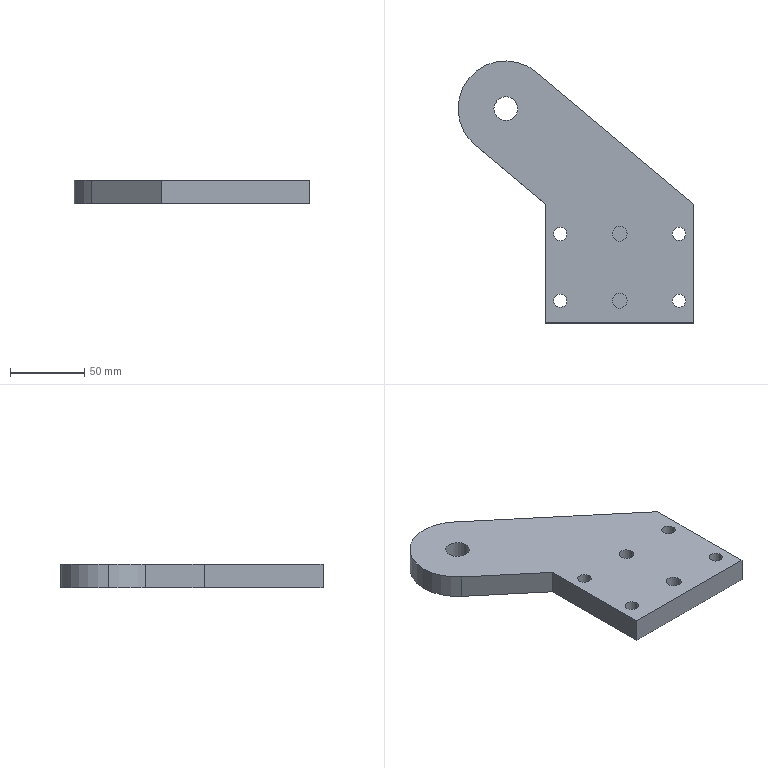Part | SolidWorks | features BaseBody 1 | 1 solid | 25 faces | box 158.743 x 176.419 x 16 mm | volume 247944 mm3 | cylinder 16 | plane 9 | commonest cylinder face diameters 9 x8 10.01 x4 16 x2 64.28 x2
STEP:
#1=CARTESIAN_POINT('',(-35.5,85.,-32.879));
#2=VERTEX_POINT('',#1);
#3=CARTESIAN_POINT('',(-44.5,85.,-32.879));
#4=VERTEX_POINT('',#3);
#5=CARTESIAN_POINT('',(-40.,85.,-32.879));
#6=DIRECTION('',(0.,0.,-1.));
#7=DIRECTION('',(1.,0.,0.));
#8=AXIS2_PLACEMENT_3D('',#5,#6,#7);
#9=CIRCLE('',#8,4.5);
#10=EDGE_CURVE('',#2,#4,#9,.T.);
#11=ORIENTED_EDGE('',*,*,#10,.T.);
#12=CARTESIAN_POINT('',(-44.5,85.,-16.879));
#13=VERTEX_POINT('',#12);
#14=CARTESIAN_POINT('',(-44.5,85.,-32.88));
#15=DIRECTION('',(0.,0.,1.));
#16=VECTOR('',#15,1000.);
#17=LINE('',#14,#16);
#18=EDGE_CURVE('',#4,#13,#17,.T.);
#19=ORIENTED_EDGE('',*,*,#18,.T.);
#20=CARTESIAN_POINT('',(-35.5,85.,-16.879));
#21=VERTEX_POINT('',#20);
#22=CARTESIAN_POINT('',(-40.,85.,-16.879));
#23=DIRECTION('',(0.,0.,-1.));
#24=DIRECTION('',(1.,0.,0.));
#25=AXIS2_PLACEMENT_3D('',#22,#23,#24);
#26=CIRCLE('',#25,4.5);
#27=EDGE_CURVE('',#21,#13,#26,.T.);
#28=ORIENTED_EDGE('',*,*,#27,.F.);
#29=CARTESIAN_POINT('',(-35.5,85.,-32.88));
#30=DIRECTION('',(0.,0.,1.));
#31=VECTOR('',#30,1000.);
#32=LINE('',#29,#31);
#33=EDGE_CURVE('',#2,#21,#32,.T.);
#34=ORIENTED_EDGE('',*,*,#33,.F.);
#35=EDGE_LOOP('',(#11,#19,#28,#34));
#36=FACE_OUTER_BOUND('',#35,.T.);
#37=CARTESIAN_POINT('',(-40.,85.,-32.88));
#38=DIRECTION('',(0.,0.,1.));
#39=DIRECTION('',(1.,0.,0.));
#40=AXIS2_PLACEMENT_3D('',#37,#38,#39);
#41=CYLINDRICAL_SURFACE('',#40,4.5);
#42=ADVANCED_FACE('',(#36),#41,.F.);
#43=CARTESIAN_POINT('',(-97.263,189.658,-16.879));
#44=VERTEX_POINT('',#43);
#45=CARTESIAN_POINT('',(-108.743,214.279,-16.879));
#46=VERTEX_POINT('',#45);
#47=CARTESIAN_POINT('',(-76.603,214.279,-16.879));
#48=DIRECTION('',(0.,0.,-1.));
#49=DIRECTION('',(-1.,0.,0.));
#50=AXIS2_PLACEMENT_3D('',#47,#48,#49);
#51=CIRCLE('',#50,32.14);
#52=EDGE_CURVE('',#44,#46,#51,.T.);
#53=ORIENTED_EDGE('',*,*,#52,.T.);
#54=CARTESIAN_POINT('',(-108.743,214.279,-32.879));
#55=VERTEX_POINT('',#54);
#56=CARTESIAN_POINT('',(-108.743,214.279,-16.879));
#57=DIRECTION('',(0.,0.,-1.));
#58=VECTOR('',#57,1000.);
#59=LINE('',#56,#58);
#60=EDGE_CURVE('',#46,#55,#59,.T.);
#61=ORIENTED_EDGE('',*,*,#60,.T.);
#62=CARTESIAN_POINT('',(-97.263,189.658,-32.879));
#63=VERTEX_POINT('',#62);
#64=CARTESIAN_POINT('',(-76.603,214.279,-32.879));
#65=DIRECTION('',(0.,0.,1.));
#66=DIRECTION('',(-1.,0.,0.));
#67=AXIS2_PLACEMENT_3D('',#64,#65,#66);
#68=CIRCLE('',#67,32.14);
#69=EDGE_CURVE('',#55,#63,#68,.T.);
#70=ORIENTED_EDGE('',*,*,#69,.T.);
#71=CARTESIAN_POINT('',(-97.263,189.658,-16.879));
#72=DIRECTION('',(0.,0.,1.));
#73=VECTOR('',#72,1000.);
#74=LINE('',#71,#73);
#75=EDGE_CURVE('',#63,#44,#74,.T.);
#76=ORIENTED_EDGE('',*,*,#75,.T.);
#77=EDGE_LOOP('',(#53,#61,#70,#76));
#78=FACE_OUTER_BOUND('',#77,.T.);
#79=CARTESIAN_POINT('',(-76.603,214.279,-16.879));
#80=DIRECTION('',(0.,0.,-1.));
#81=DIRECTION('',(-1.,0.,0.));
#82=AXIS2_PLACEMENT_3D('',#79,#80,#81);
#83=CYLINDRICAL_SURFACE('',#82,32.14);
#84=ADVANCED_FACE('',(#78),#83,.T.);
#85=CARTESIAN_POINT('',(44.5,130.,-32.879));
#86=VERTEX_POINT('',#85);
#87=CARTESIAN_POINT('',(35.5,130.,-32.879));
#88=VERTEX_POINT('',#87);
#89=CARTESIAN_POINT('',(40.,130.,-32.879));
#90=DIRECTION('',(0.,0.,-1.));
#91=DIRECTION('',(1.,0.,0.));
#92=AXIS2_PLACEMENT_3D('',#89,#90,#91);
#93=CIRCLE('',#92,4.5);
#94=EDGE_CURVE('',#86,#88,#93,.T.);
#95=ORIENTED_EDGE('',*,*,#94,.T.);
#96=CARTESIAN_POINT('',(35.5,130.,-16.879));
#97=VERTEX_POINT('',#96);
#98=CARTESIAN_POINT('',(35.5,130.,-32.88));
#99=DIRECTION('',(0.,0.,1.));
#100=VECTOR('',#99,1000.);
#101=LINE('',#98,#100);
#102=EDGE_CURVE('',#88,#97,#101,.T.);
#103=ORIENTED_EDGE('',*,*,#102,.T.);
#104=CARTESIAN_POINT('',(44.5,130.,-16.879));
#105=VERTEX_POINT('',#104);
#106=CARTESIAN_POINT('',(40.,130.,-16.879));
#107=DIRECTION('',(0.,0.,-1.));
#108=DIRECTION('',(1.,0.,0.));
#109=AXIS2_PLACEMENT_3D('',#106,#107,#108);
#110=CIRCLE('',#109,4.5);
#111=EDGE_CURVE('',#105,#97,#110,.T.);
#112=ORIENTED_EDGE('',*,*,#111,.F.);
#113=CARTESIAN_POINT('',(44.5,130.,-32.88));
#114=DIRECTION('',(0.,0.,1.));
#115=VECTOR('',#114,1000.);
#116=LINE('',#113,#115);
#117=EDGE_CURVE('',#86,#105,#116,.T.);
#118=ORIENTED_EDGE('',*,*,#117,.F.);
#119=EDGE_LOOP('',(#95,#103,#112,#118));
#120=FACE_OUTER_BOUND('',#119,.T.);
#121=CARTESIAN_POINT('',(40.,130.,-32.88));
#122=DIRECTION('',(0.,0.,1.));
#123=DIRECTION('',(1.,0.,0.));
#124=AXIS2_PLACEMENT_3D('',#121,#122,#123);
#125=CYLINDRICAL_SURFACE('',#124,4.5);
#126=ADVANCED_FACE('',(#120),#125,.F.);
#127=CARTESIAN_POINT('',(44.5,85.,-32.879));
#128=VERTEX_POINT('',#127);
#129=CARTESIAN_POINT('',(35.5,85.,-32.879));
#130=VERTEX_POINT('',#129);
#131=CARTESIAN_POINT('',(40.,85.,-32.879));
#132=DIRECTION('',(0.,0.,-1.));
#133=DIRECTION('',(1.,0.,0.));
#134=AXIS2_PLACEMENT_3D('',#131,#132,#133);
#135=CIRCLE('',#134,4.5);
#136=EDGE_CURVE('',#128,#130,#135,.T.);
#137=ORIENTED_EDGE('',*,*,#136,.T.);
#138=CARTESIAN_POINT('',(35.5,85.,-16.879));
#139=VERTEX_POINT('',#138);
#140=CARTESIAN_POINT('',(35.5,85.,-32.88));
#141=DIRECTION('',(0.,0.,1.));
#142=VECTOR('',#141,1000.);
#143=LINE('',#140,#142);
#144=EDGE_CURVE('',#130,#139,#143,.T.);
#145=ORIENTED_EDGE('',*,*,#144,.T.);
#146=CARTESIAN_POINT('',(44.5,85.,-16.879));
#147=VERTEX_POINT('',#146);
#148=CARTESIAN_POINT('',(40.,85.,-16.879));
#149=DIRECTION('',(0.,0.,-1.));
#150=DIRECTION('',(1.,0.,0.));
#151=AXIS2_PLACEMENT_3D('',#148,#149,#150);
#152=CIRCLE('',#151,4.5);
#153=EDGE_CURVE('',#147,#139,#152,.T.);
#154=ORIENTED_EDGE('',*,*,#153,.F.);
#155=CARTESIAN_POINT('',(44.5,85.,-32.88));
#156=DIRECTION('',(0.,0.,1.));
#157=VECTOR('',#156,1000.);
#158=LINE('',#155,#157);
#159=EDGE_CURVE('',#128,#147,#158,.T.);
#160=ORIENTED_EDGE('',*,*,#159,.F.);
#161=EDGE_LOOP('',(#137,#145,#154,#160));
#162=FACE_OUTER_BOUND('',#161,.T.);
#163=CARTESIAN_POINT('',(40.,85.,-32.88));
#164=DIRECTION('',(0.,0.,1.));
#165=DIRECTION('',(1.,0.,0.));
#166=AXIS2_PLACEMENT_3D('',#163,#164,#165);
#167=CYLINDRICAL_SURFACE('',#166,4.5);
#168=ADVANCED_FACE('',(#162),#167,.F.);
#169=CARTESIAN_POINT('',(-35.5,130.,-32.879));
#170=VERTEX_POINT('',#169);
#171=CARTESIAN_POINT('',(-44.5,130.,-32.879));
#172=VERTEX_POINT('',#171);
#173=CARTESIAN_POINT('',(-40.,130.,-32.879));
#174=DIRECTION('',(0.,0.,-1.));
#175=DIRECTION('',(1.,0.,0.));
#176=AXIS2_PLACEMENT_3D('',#173,#174,#175);
#177=CIRCLE('',#176,4.5);
#178=EDGE_CURVE('',#170,#172,#177,.T.);
#179=ORIENTED_EDGE('',*,*,#178,.T.);
#180=CARTESIAN_POINT('',(-44.5,130.,-16.879));
#181=VERTEX_POINT('',#180);
#182=CARTESIAN_POINT('',(-44.5,130.,-32.88));
#183=DIRECTION('',(0.,0.,1.));
#184=VECTOR('',#183,1000.);
#185=LINE('',#182,#184);
#186=EDGE_CURVE('',#172,#181,#185,.T.);
#187=ORIENTED_EDGE('',*,*,#186,.T.);
#188=CARTESIAN_POINT('',(-35.5,130.,-16.879));
#189=VERTEX_POINT('',#188);
#190=CARTESIAN_POINT('',(-40.,130.,-16.879));
#191=DIRECTION('',(0.,0.,-1.));
#192=DIRECTION('',(1.,0.,0.));
#193=AXIS2_PLACEMENT_3D('',#190,#191,#192);
#194=CIRCLE('',#193,4.5);
#195=EDGE_CURVE('',#189,#181,#194,.T.);
#196=ORIENTED_EDGE('',*,*,#195,.F.);
#197=CARTESIAN_POINT('',(-35.5,130.,-32.88));
#198=DIRECTION('',(0.,0.,1.));
#199=VECTOR('',#198,1000.);
#200=LINE('',#197,#199);
#201=EDGE_CURVE('',#170,#189,#200,.T.);
#202=ORIENTED_EDGE('',*,*,#201,.F.);
#203=EDGE_LOOP('',(#179,#187,#196,#202));
#204=FACE_OUTER_BOUND('',#203,.T.);
#205=CARTESIAN_POINT('',(-40.,130.,-32.88));
#206=DIRECTION('',(0.,0.,1.));
#207=DIRECTION('',(1.,0.,0.));
#208=AXIS2_PLACEMENT_3D('',#205,#206,#207);
#209=CYLINDRICAL_SURFACE('',#208,4.5);
#210=ADVANCED_FACE('',(#204),#209,.F.);
#211=CARTESIAN_POINT('',(-68.603,214.279,-32.879));
#212=VERTEX_POINT('',#211);
#213=CARTESIAN_POINT('',(-84.603,214.279,-32.879));
#214=VERTEX_POINT('',#213);
#215=CARTESIAN_POINT('',(-76.603,214.279,-32.879));
#216=DIRECTION('',(0.,0.,-1.));
#217=DIRECTION('',(1.,0.,0.));
#218=AXIS2_PLACEMENT_3D('',#215,#216,#217);
#219=CIRCLE('',#218,8.);
#220=EDGE_CURVE('',#212,#214,#219,.T.);
#221=ORIENTED_EDGE('',*,*,#220,.T.);
#222=CARTESIAN_POINT('',(-84.603,214.279,-16.879));
#223=VERTEX_POINT('',#222);
#224=CARTESIAN_POINT('',(-84.603,214.279,-32.88));
#225=DIRECTION('',(0.,0.,1.));
#226=VECTOR('',#225,1000.);
#227=LINE('',#224,#226);
#228=EDGE_CURVE('',#214,#223,#227,.T.);
#229=ORIENTED_EDGE('',*,*,#228,.T.);
#230=CARTESIAN_POINT('',(-68.603,214.279,-16.879));
#231=VERTEX_POINT('',#230);
#232=CARTESIAN_POINT('',(-76.603,214.279,-16.879));
#233=DIRECTION('',(0.,0.,-1.));
#234=DIRECTION('',(1.,0.,0.));
#235=AXIS2_PLACEMENT_3D('',#232,#233,#234);
#236=CIRCLE('',#235,8.);
#237=EDGE_CURVE('',#231,#223,#236,.T.);
#238=ORIENTED_EDGE('',*,*,#237,.F.);
#239=CARTESIAN_POINT('',(-68.603,214.279,-32.88));
#240=DIRECTION('',(0.,0.,1.));
#241=VECTOR('',#240,1000.);
#242=LINE('',#239,#241);
#243=EDGE_CURVE('',#212,#231,#242,.T.);
#244=ORIENTED_EDGE('',*,*,#243,.F.);
#245=EDGE_LOOP('',(#221,#229,#238,#244));
#246=FACE_OUTER_BOUND('',#245,.T.);
#247=CARTESIAN_POINT('',(-76.603,214.279,-32.88));
#248=DIRECTION('',(0.,0.,1.));
#249=DIRECTION('',(1.,0.,0.));
#250=AXIS2_PLACEMENT_3D('',#247,#248,#249);
#251=CYLINDRICAL_SURFACE('',#250,8.);
#252=ADVANCED_FACE('',(#246),#251,.F.);
#253=CARTESIAN_POINT('',(-5.005,130.,-26.879));
#254=VERTEX_POINT('',#253);
#255=CARTESIAN_POINT('',(5.005,130.,-26.879));
#256=VERTEX_POINT('',#255);
#257=CARTESIAN_POINT('',(0.,130.,-26.879));
#258=DIRECTION('',(0.,0.,1.));
#259=DIRECTION('',(1.,0.,0.));
#260=AXIS2_PLACEMENT_3D('',#257,#258,#259);
#261=CIRCLE('',#260,5.005);
#262=EDGE_CURVE('',#254,#256,#261,.T.);
#263=ORIENTED_EDGE('',*,*,#262,.F.);
#264=CARTESIAN_POINT('',(-5.005,130.,-16.879));
#265=VERTEX_POINT('',#264);
#266=CARTESIAN_POINT('',(-5.005,130.,-26.879));
#267=DIRECTION('',(0.,0.,1.));
#268=VECTOR('',#267,1000.);
#269=LINE('',#266,#268);
#270=EDGE_CURVE('',#254,#265,#269,.T.);
#271=ORIENTED_EDGE('',*,*,#270,.T.);
#272=CARTESIAN_POINT('',(5.005,130.,-16.879));
#273=VERTEX_POINT('',#272);
#274=CARTESIAN_POINT('',(0.,130.,-16.879));
#275=DIRECTION('',(0.,0.,-1.));
#276=DIRECTION('',(1.,0.,0.));
#277=AXIS2_PLACEMENT_3D('',#274,#275,#276);
#278=CIRCLE('',#277,5.005);
#279=EDGE_CURVE('',#273,#265,#278,.T.);
#280=ORIENTED_EDGE('',*,*,#279,.F.);
#281=CARTESIAN_POINT('',(5.005,130.,-26.879));
#282=DIRECTION('',(0.,0.,1.));
#283=VECTOR('',#282,1000.);
#284=LINE('',#281,#283);
#285=EDGE_CURVE('',#256,#273,#284,.T.);
#286=ORIENTED_EDGE('',*,*,#285,.F.);
#287=EDGE_LOOP('',(#263,#271,#280,#286));
#288=FACE_OUTER_BOUND('',#287,.T.);
#289=CARTESIAN_POINT('',(0.,130.,-26.879));
#290=DIRECTION('',(0.,0.,1.));
#291=DIRECTION('',(1.,0.,0.));
#292=AXIS2_PLACEMENT_3D('',#289,#290,#291);
#293=CYLINDRICAL_SURFACE('',#292,5.005);
#294=ADVANCED_FACE('',(#288),#293,.F.);
#295=CARTESIAN_POINT('',(-5.005,85.,-26.879));
#296=VERTEX_POINT('',#295);
#297=CARTESIAN_POINT('',(5.005,85.,-26.879));
#298=VERTEX_POINT('',#297);
#299=CARTESIAN_POINT('',(0.,85.,-26.879));
#300=DIRECTION('',(0.,0.,1.));
#301=DIRECTION('',(1.,0.,0.));
#302=AXIS2_PLACEMENT_3D('',#299,#300,#301);
#303=CIRCLE('',#302,5.005);
#304=EDGE_CURVE('',#296,#298,#303,.T.);
#305=ORIENTED_EDGE('',*,*,#304,.F.);
#306=CARTESIAN_POINT('',(-5.005,85.,-16.879));
#307=VERTEX_POINT('',#306);
#308=CARTESIAN_POINT('',(-5.005,85.,-26.879));
#309=DIRECTION('',(0.,0.,1.));
#310=VECTOR('',#309,1000.);
#311=LINE('',#308,#310);
#312=EDGE_CURVE('',#296,#307,#311,.T.);
#313=ORIENTED_EDGE('',*,*,#312,.T.);
#314=CARTESIAN_POINT('',(5.005,85.,-16.879));
#315=VERTEX_POINT('',#314);
#316=CARTESIAN_POINT('',(0.,85.,-16.879));
#317=DIRECTION('',(0.,0.,-1.));
#318=DIRECTION('',(1.,0.,0.));
#319=AXIS2_PLACEMENT_3D('',#316,#317,#318);
#320=CIRCLE('',#319,5.005);
#321=EDGE_CURVE('',#315,#307,#320,.T.);
#322=ORIENTED_EDGE('',*,*,#321,.F.);
#323=CARTESIAN_POINT('',(5.005,85.,-26.879));
#324=DIRECTION('',(0.,0.,1.));
#325=VECTOR('',#324,1000.);
#326=LINE('',#323,#325);
#327=EDGE_CURVE('',#298,#315,#326,.T.);
#328=ORIENTED_EDGE('',*,*,#327,.F.);
#329=EDGE_LOOP('',(#305,#313,#322,#328));
#330=FACE_OUTER_BOUND('',#329,.T.);
#331=CARTESIAN_POINT('',(0.,85.,-26.879));
#332=DIRECTION('',(0.,0.,1.));
#333=DIRECTION('',(1.,0.,0.));
#334=AXIS2_PLACEMENT_3D('',#331,#332,#333);
#335=CYLINDRICAL_SURFACE('',#334,5.005);
#336=ADVANCED_FACE('',(#330),#335,.F.);
#337=ORIENTED_EDGE('',*,*,#10,.F.);
#338=CARTESIAN_POINT('',(-40.,85.,-32.879));
#339=DIRECTION('',(0.,0.,-1.));
#340=DIRECTION('',(1.,0.,0.));
#341=AXIS2_PLACEMENT_3D('',#338,#339,#340);
#342=CIRCLE('',#341,4.5);
#343=EDGE_CURVE('',#4,#2,#342,.T.);
#344=ORIENTED_EDGE('',*,*,#343,.F.);
#345=EDGE_LOOP('',(#337,#344));
#346=FACE_BOUND('',#345,.T.);
#347=CARTESIAN_POINT('',(-50.,70.,-32.879));
#348=VERTEX_POINT('',#347);
#349=CARTESIAN_POINT('',(50.,70.,-32.879));
#350=VERTEX_POINT('',#349);
#351=CARTESIAN_POINT('',(-76.603,70.,-32.879));
#352=DIRECTION('',(1.,0.,0.));
#353=VECTOR('',#352,1000.);
#354=LINE('',#351,#353);
#355=EDGE_CURVE('',#348,#350,#354,.T.);
#356=ORIENTED_EDGE('',*,*,#355,.F.);
#357=CARTESIAN_POINT('',(-50.,150.,-32.879));
#358=VERTEX_POINT('',#357);
#359=CARTESIAN_POINT('',(-50.,214.279,-32.879));
#360=DIRECTION('',(0.,-1.,0.));
#361=VECTOR('',#360,1000.);
#362=LINE('',#359,#361);
#363=EDGE_CURVE('',#358,#348,#362,.T.);
#364=ORIENTED_EDGE('',*,*,#363,.F.);
#365=CARTESIAN_POINT('',(-97.263,189.658,-32.879));
#366=DIRECTION('',(0.766,-0.6428,0.));
#367=VECTOR('',#366,1000.);
#368=LINE('',#365,#367);
#369=EDGE_CURVE('',#63,#358,#368,.T.);
#370=ORIENTED_EDGE('',*,*,#369,.F.);
#371=ORIENTED_EDGE('',*,*,#69,.F.);
#372=CARTESIAN_POINT('',(-55.729,238.717,-32.879));
#373=VERTEX_POINT('',#372);
#374=CARTESIAN_POINT('',(-76.603,214.279,-32.879));
#375=DIRECTION('',(0.,0.,1.));
#376=DIRECTION('',(-1.,0.,0.));
#377=AXIS2_PLACEMENT_3D('',#374,#375,#376);
#378=CIRCLE('',#377,32.14);
#379=EDGE_CURVE('',#373,#55,#378,.T.);
#380=ORIENTED_EDGE('',*,*,#379,.F.);
#381=CARTESIAN_POINT('',(50.,150.,-32.879));
#382=VERTEX_POINT('',#381);
#383=CARTESIAN_POINT('',(50.,150.,-32.879));
#384=DIRECTION('',(-0.766,0.6428,0.));
#385=VECTOR('',#384,1000.);
#386=LINE('',#383,#385);
#387=EDGE_CURVE('',#382,#373,#386,.T.);
#388=ORIENTED_EDGE('',*,*,#387,.F.);
#389=CARTESIAN_POINT('',(50.,214.279,-32.879));
#390=DIRECTION('',(0.,1.,0.));
#391=VECTOR('',#390,1000.);
#392=LINE('',#389,#391);
#393=EDGE_CURVE('',#350,#382,#392,.T.);
#394=ORIENTED_EDGE('',*,*,#393,.F.);
#395=EDGE_LOOP('',(#356,#364,#370,#371,#380,#388,#394));
#396=FACE_OUTER_BOUND('',#395,.T.);
#397=ORIENTED_EDGE('',*,*,#94,.F.);
#398=CARTESIAN_POINT('',(40.,130.,-32.879));
#399=DIRECTION('',(0.,0.,-1.));
#400=DIRECTION('',(1.,0.,0.));
#401=AXIS2_PLACEMENT_3D('',#398,#399,#400);
#402=CIRCLE('',#401,4.5);
#403=EDGE_CURVE('',#88,#86,#402,.T.);
#404=ORIENTED_EDGE('',*,*,#403,.F.);
#405=EDGE_LOOP('',(#397,#404));
#406=FACE_BOUND('',#405,.T.);
#407=ORIENTED_EDGE('',*,*,#136,.F.);
#408=CARTESIAN_POINT('',(40.,85.,-32.879));
#409=DIRECTION('',(0.,0.,-1.));
#410=DIRECTION('',(1.,0.,0.));
#411=AXIS2_PLACEMENT_3D('',#408,#409,#410);
#412=CIRCLE('',#411,4.5);
#413=EDGE_CURVE('',#130,#128,#412,.T.);
#414=ORIENTED_EDGE('',*,*,#413,.F.);
#415=EDGE_LOOP('',(#407,#414));
#416=FACE_BOUND('',#415,.T.);
#417=ORIENTED_EDGE('',*,*,#178,.F.);
#418=CARTESIAN_POINT('',(-40.,130.,-32.879));
#419=DIRECTION('',(0.,0.,-1.));
#420=DIRECTION('',(1.,0.,0.));
#421=AXIS2_PLACEMENT_3D('',#418,#419,#420);
#422=CIRCLE('',#421,4.5);
#423=EDGE_CURVE('',#172,#170,#422,.T.);
#424=ORIENTED_EDGE('',*,*,#423,.F.);
#425=EDGE_LOOP('',(#417,#424));
#426=FACE_BOUND('',#425,.T.);
#427=ORIENTED_EDGE('',*,*,#220,.F.);
#428=CARTESIAN_POINT('',(-76.603,214.279,-32.879));
#429=DIRECTION('',(0.,0.,-1.));
#430=DIRECTION('',(1.,0.,0.));
#431=AXIS2_PLACEMENT_3D('',#428,#429,#430);
#432=CIRCLE('',#431,8.);
#433=EDGE_CURVE('',#214,#212,#432,.T.);
#434=ORIENTED_EDGE('',*,*,#433,.F.);
#435=EDGE_LOOP('',(#427,#434));
#436=FACE_BOUND('',#435,.T.);
#437=CARTESIAN_POINT('',(-76.603,214.279,-32.879));
#438=DIRECTION('',(0.,0.,1.));
#439=DIRECTION('',(1.,0.,0.));
#440=AXIS2_PLACEMENT_3D('',#437,#438,#439);
#441=PLANE('',#440);
#442=ADVANCED_FACE('',(#346,#396,#406,#416,#426,#436),#441,.F.);
#443=ORIENTED_EDGE('',*,*,#18,.F.);
#444=ORIENTED_EDGE('',*,*,#343,.T.);
#445=ORIENTED_EDGE('',*,*,#33,.T.);
#446=CARTESIAN_POINT('',(-40.,85.,-16.879));
#447=DIRECTION('',(0.,0.,-1.));
#448=DIRECTION('',(1.,0.,0.));
#449=AXIS2_PLACEMENT_3D('',#446,#447,#448);
#450=CIRCLE('',#449,4.5);
#451=EDGE_CURVE('',#13,#21,#450,.T.);
#452=ORIENTED_EDGE('',*,*,#451,.F.);
#453=EDGE_LOOP('',(#443,#444,#445,#452));
#454=FACE_OUTER_BOUND('',#453,.T.);
#455=CARTESIAN_POINT('',(-40.,85.,-32.88));
#456=DIRECTION('',(0.,0.,1.));
#457=DIRECTION('',(1.,0.,0.));
#458=AXIS2_PLACEMENT_3D('',#455,#456,#457);
#459=CYLINDRICAL_SURFACE('',#458,4.5);
#460=ADVANCED_FACE('',(#454),#459,.F.);
#461=CARTESIAN_POINT('',(50.,150.,-16.879));
#462=VERTEX_POINT('',#461);
#463=CARTESIAN_POINT('',(50.,150.,-16.879));
#464=DIRECTION('',(0.,0.,-1.));
#465=VECTOR('',#464,1000.);
#466=LINE('',#463,#465);
#467=EDGE_CURVE('',#462,#382,#466,.T.);
#468=ORIENTED_EDGE('',*,*,#467,.F.);
#469=CARTESIAN_POINT('',(50.,70.,-16.879));
#470=VERTEX_POINT('',#469);
#471=CARTESIAN_POINT('',(50.,70.,-16.879));
#472=DIRECTION('',(0.,1.,0.));
#473=VECTOR('',#472,1000.);
#474=LINE('',#471,#473);
#475=EDGE_CURVE('',#470,#462,#474,.T.);
#476=ORIENTED_EDGE('',*,*,#475,.F.);
#477=CARTESIAN_POINT('',(50.,70.,-16.879));
#478=DIRECTION('',(0.,0.,1.));
#479=VECTOR('',#478,1000.);
#480=LINE('',#477,#479);
#481=EDGE_CURVE('',#350,#470,#480,.T.);
#482=ORIENTED_EDGE('',*,*,#481,.F.);
#483=ORIENTED_EDGE('',*,*,#393,.T.);
#484=EDGE_LOOP('',(#468,#476,#482,#483));
#485=FACE_OUTER_BOUND('',#484,.T.);
#486=CARTESIAN_POINT('',(50.,70.,-16.879));
#487=DIRECTION('',(-1.,0.,0.));
#488=DIRECTION('',(0.,0.,1.));
#489=AXIS2_PLACEMENT_3D('',#486,#487,#488);
#490=PLANE('',#489);
#491=ADVANCED_FACE('',(#485),#490,.F.);
#492=ORIENTED_EDGE('',*,*,#481,.T.);
#493=CARTESIAN_POINT('',(-50.,70.,-16.879));
#494=VERTEX_POINT('',#493);
#495=CARTESIAN_POINT('',(-50.,70.,-16.879));
#496=DIRECTION('',(1.,0.,0.));
#497=VECTOR('',#496,1000.);
#498=LINE('',#495,#497);
#499=EDGE_CURVE('',#494,#470,#498,.T.);
#500=ORIENTED_EDGE('',*,*,#499,.F.);
#501=CARTESIAN_POINT('',(-50.,70.,-16.879));
#502=DIRECTION('',(0.,0.,1.));
#503=VECTOR('',#502,1000.);
#504=LINE('',#501,#503);
#505=EDGE_CURVE('',#348,#494,#504,.T.);
#506=ORIENTED_EDGE('',*,*,#505,.F.);
#507=ORIENTED_EDGE('',*,*,#355,.T.);
#508=EDGE_LOOP('',(#492,#500,#506,#507));
#509=FACE_OUTER_BOUND('',#508,.T.);
#510=CARTESIAN_POINT('',(-50.,70.,-16.879));
#511=DIRECTION('',(0.,1.,0.));
#512=DIRECTION('',(0.,0.,1.));
#513=AXIS2_PLACEMENT_3D('',#510,#511,#512);
#514=PLANE('',#513);
#515=ADVANCED_FACE('',(#509),#514,.F.);
#516=ORIENTED_EDGE('',*,*,#505,.T.);
#517=CARTESIAN_POINT('',(-50.,150.,-16.879));
#518=VERTEX_POINT('',#517);
#519=CARTESIAN_POINT('',(-50.,70.,-16.879));
#520=DIRECTION('',(0.,-1.,0.));
#521=VECTOR('',#520,1000.);
#522=LINE('',#519,#521);
#523=EDGE_CURVE('',#518,#494,#522,.T.);
#524=ORIENTED_EDGE('',*,*,#523,.F.);
#525=CARTESIAN_POINT('',(-50.,150.,-16.879));
#526=DIRECTION('',(0.,0.,1.));
#527=VECTOR('',#526,1000.);
#528=LINE('',#525,#527);
#529=EDGE_CURVE('',#358,#518,#528,.T.);
#530=ORIENTED_EDGE('',*,*,#529,.F.);
#531=ORIENTED_EDGE('',*,*,#363,.T.);
#532=EDGE_LOOP('',(#516,#524,#530,#531));
#533=FACE_OUTER_BOUND('',#532,.T.);
#534=CARTESIAN_POINT('',(-50.,70.,-16.879));
#535=DIRECTION('',(1.,0.,0.));
#536=DIRECTION('',(0.,0.,-1.));
#537=AXIS2_PLACEMENT_3D('',#534,#535,#536);
#538=PLANE('',#537);
#539=ADVANCED_FACE('',(#533),#538,.F.);
#540=ORIENTED_EDGE('',*,*,#529,.T.);
#541=CARTESIAN_POINT('',(-50.,150.,-16.879));
#542=DIRECTION('',(0.766,-0.6428,0.));
#543=VECTOR('',#542,1000.);
#544=LINE('',#541,#543);
#545=EDGE_CURVE('',#44,#518,#544,.T.);
#546=ORIENTED_EDGE('',*,*,#545,.F.);
#547=ORIENTED_EDGE('',*,*,#75,.F.);
#548=ORIENTED_EDGE('',*,*,#369,.T.);
#549=EDGE_LOOP('',(#540,#546,#547,#548));
#550=FACE_OUTER_BOUND('',#549,.T.);
#551=CARTESIAN_POINT('',(-50.,150.,-16.879));
#552=DIRECTION('',(0.6428,0.766,0.));
#553=DIRECTION('',(-0.766,0.6428,0.));
#554=AXIS2_PLACEMENT_3D('',#551,#552,#553);
#555=PLANE('',#554);
#556=ADVANCED_FACE('',(#550),#555,.F.);
#557=ORIENTED_EDGE('',*,*,#60,.F.);
#558=CARTESIAN_POINT('',(-55.729,238.717,-16.879));
#559=VERTEX_POINT('',#558);
#560=CARTESIAN_POINT('',(-76.603,214.279,-16.879));
#561=DIRECTION('',(0.,0.,-1.));
#562=DIRECTION('',(-1.,0.,0.));
#563=AXIS2_PLACEMENT_3D('',#560,#561,#562);
#564=CIRCLE('',#563,32.14);
#565=EDGE_CURVE('',#46,#559,#564,.T.);
#566=ORIENTED_EDGE('',*,*,#565,.T.);
#567=CARTESIAN_POINT('',(-55.729,238.717,-16.879));
#568=DIRECTION('',(0.,0.,-1.));
#569=VECTOR('',#568,1000.);
#570=LINE('',#567,#569);
#571=EDGE_CURVE('',#559,#373,#570,.T.);
#572=ORIENTED_EDGE('',*,*,#571,.T.);
#573=ORIENTED_EDGE('',*,*,#379,.T.);
#574=EDGE_LOOP('',(#557,#566,#572,#573));
#575=FACE_OUTER_BOUND('',#574,.T.);
#576=CARTESIAN_POINT('',(-76.603,214.279,-16.879));
#577=DIRECTION('',(0.,0.,-1.));
#578=DIRECTION('',(-1.,0.,0.));
#579=AXIS2_PLACEMENT_3D('',#576,#577,#578);
#580=CYLINDRICAL_SURFACE('',#579,32.14);
#581=ADVANCED_FACE('',(#575),#580,.T.);
#582=ORIENTED_EDGE('',*,*,#571,.F.);
#583=CARTESIAN_POINT('',(50.,150.,-16.879));
#584=DIRECTION('',(-0.766,0.6428,0.));
#585=VECTOR('',#584,1000.);
#586=LINE('',#583,#585);
#587=EDGE_CURVE('',#462,#559,#586,.T.);
#588=ORIENTED_EDGE('',*,*,#587,.F.);
#589=ORIENTED_EDGE('',*,*,#467,.T.);
#590=ORIENTED_EDGE('',*,*,#387,.T.);
#591=EDGE_LOOP('',(#582,#588,#589,#590));
#592=FACE_OUTER_BOUND('',#591,.T.);
#593=CARTESIAN_POINT('',(50.,150.,-16.879));
#594=DIRECTION('',(-0.6428,-0.766,0.));
#595=DIRECTION('',(0.766,-0.6428,0.));
#596=AXIS2_PLACEMENT_3D('',#593,#594,#595);
#597=PLANE('',#596);
#598=ADVANCED_FACE('',(#592),#597,.F.);
#599=ORIENTED_EDGE('',*,*,#102,.F.);
#600=ORIENTED_EDGE('',*,*,#403,.T.);
#601=ORIENTED_EDGE('',*,*,#117,.T.);
#602=CARTESIAN_POINT('',(40.,130.,-16.879));
#603=DIRECTION('',(0.,0.,-1.));
#604=DIRECTION('',(1.,0.,0.));
#605=AXIS2_PLACEMENT_3D('',#602,#603,#604);
#606=CIRCLE('',#605,4.5);
#607=EDGE_CURVE('',#97,#105,#606,.T.);
#608=ORIENTED_EDGE('',*,*,#607,.F.);
#609=EDGE_LOOP('',(#599,#600,#601,#608));
#610=FACE_OUTER_BOUND('',#609,.T.);
#611=CARTESIAN_POINT('',(40.,130.,-32.88));
#612=DIRECTION('',(0.,0.,1.));
#613=DIRECTION('',(1.,0.,0.));
#614=AXIS2_PLACEMENT_3D('',#611,#612,#613);
#615=CYLINDRICAL_SURFACE('',#614,4.5);
#616=ADVANCED_FACE('',(#610),#615,.F.);
#617=ORIENTED_EDGE('',*,*,#144,.F.);
#618=ORIENTED_EDGE('',*,*,#413,.T.);
#619=ORIENTED_EDGE('',*,*,#159,.T.);
#620=CARTESIAN_POINT('',(40.,85.,-16.879));
#621=DIRECTION('',(0.,0.,-1.));
#622=DIRECTION('',(1.,0.,0.));
#623=AXIS2_PLACEMENT_3D('',#620,#621,#622);
#624=CIRCLE('',#623,4.5);
#625=EDGE_CURVE('',#139,#147,#624,.T.);
#626=ORIENTED_EDGE('',*,*,#625,.F.);
#627=EDGE_LOOP('',(#617,#618,#619,#626));
#628=FACE_OUTER_BOUND('',#627,.T.);
#629=CARTESIAN_POINT('',(40.,85.,-32.88));
#630=DIRECTION('',(0.,0.,1.));
#631=DIRECTION('',(1.,0.,0.));
#632=AXIS2_PLACEMENT_3D('',#629,#630,#631);
#633=CYLINDRICAL_SURFACE('',#632,4.5);
#634=ADVANCED_FACE('',(#628),#633,.F.);
#635=ORIENTED_EDGE('',*,*,#186,.F.);
#636=ORIENTED_EDGE('',*,*,#423,.T.);
#637=ORIENTED_EDGE('',*,*,#201,.T.);
#638=CARTESIAN_POINT('',(-40.,130.,-16.879));
#639=DIRECTION('',(0.,0.,-1.));
#640=DIRECTION('',(1.,0.,0.));
#641=AXIS2_PLACEMENT_3D('',#638,#639,#640);
#642=CIRCLE('',#641,4.5);
#643=EDGE_CURVE('',#181,#189,#642,.T.);
#644=ORIENTED_EDGE('',*,*,#643,.F.);
#645=EDGE_LOOP('',(#635,#636,#637,#644));
#646=FACE_OUTER_BOUND('',#645,.T.);
#647=CARTESIAN_POINT('',(-40.,130.,-32.88));
#648=DIRECTION('',(0.,0.,1.));
#649=DIRECTION('',(1.,0.,0.));
#650=AXIS2_PLACEMENT_3D('',#647,#648,#649);
#651=CYLINDRICAL_SURFACE('',#650,4.5);
#652=ADVANCED_FACE('',(#646),#651,.F.);
#653=ORIENTED_EDGE('',*,*,#228,.F.);
#654=ORIENTED_EDGE('',*,*,#433,.T.);
#655=ORIENTED_EDGE('',*,*,#243,.T.);
#656=CARTESIAN_POINT('',(-76.603,214.279,-16.879));
#657=DIRECTION('',(0.,0.,-1.));
#658=DIRECTION('',(1.,0.,0.));
#659=AXIS2_PLACEMENT_3D('',#656,#657,#658);
#660=CIRCLE('',#659,8.);
#661=EDGE_CURVE('',#223,#231,#660,.T.);
#662=ORIENTED_EDGE('',*,*,#661,.F.);
#663=EDGE_LOOP('',(#653,#654,#655,#662));
#664=FACE_OUTER_BOUND('',#663,.T.);
#665=CARTESIAN_POINT('',(-76.603,214.279,-32.88));
#666=DIRECTION('',(0.,0.,1.));
#667=DIRECTION('',(1.,0.,0.));
#668=AXIS2_PLACEMENT_3D('',#665,#666,#667);
#669=CYLINDRICAL_SURFACE('',#668,8.);
#670=ADVANCED_FACE('',(#664),#669,.F.);
#671=ORIENTED_EDGE('',*,*,#27,.T.);
#672=ORIENTED_EDGE('',*,*,#451,.T.);
#673=EDGE_LOOP('',(#671,#672));
#674=FACE_BOUND('',#673,.T.);
#675=ORIENTED_EDGE('',*,*,#523,.T.);
#676=ORIENTED_EDGE('',*,*,#499,.T.);
#677=ORIENTED_EDGE('',*,*,#475,.T.);
#678=ORIENTED_EDGE('',*,*,#587,.T.);
#679=ORIENTED_EDGE('',*,*,#565,.F.);
#680=ORIENTED_EDGE('',*,*,#52,.F.);
#681=ORIENTED_EDGE('',*,*,#545,.T.);
#682=EDGE_LOOP('',(#675,#676,#677,#678,#679,#680,#681));
#683=FACE_OUTER_BOUND('',#682,.T.);
#684=ORIENTED_EDGE('',*,*,#111,.T.);
#685=ORIENTED_EDGE('',*,*,#607,.T.);
#686=EDGE_LOOP('',(#684,#685));
#687=FACE_BOUND('',#686,.T.);
#688=ORIENTED_EDGE('',*,*,#153,.T.);
#689=ORIENTED_EDGE('',*,*,#625,.T.);
#690=EDGE_LOOP('',(#688,#689));
#691=FACE_BOUND('',#690,.T.);
#692=ORIENTED_EDGE('',*,*,#195,.T.);
#693=ORIENTED_EDGE('',*,*,#643,.T.);
#694=EDGE_LOOP('',(#692,#693));
#695=FACE_BOUND('',#694,.T.);
#696=ORIENTED_EDGE('',*,*,#237,.T.);
#697=ORIENTED_EDGE('',*,*,#661,.T.);
#698=EDGE_LOOP('',(#696,#697));
#699=FACE_BOUND('',#698,.T.);
#700=ORIENTED_EDGE('',*,*,#279,.T.);
#701=CARTESIAN_POINT('',(0.,130.,-16.879));
#702=DIRECTION('',(0.,0.,-1.));
#703=DIRECTION('',(1.,0.,0.));
#704=AXIS2_PLACEMENT_3D('',#701,#702,#703);
#705=CIRCLE('',#704,5.005);
#706=EDGE_CURVE('',#265,#273,#705,.T.);
#707=ORIENTED_EDGE('',*,*,#706,.T.);
#708=EDGE_LOOP('',(#700,#707));
#709=FACE_BOUND('',#708,.T.);
#710=ORIENTED_EDGE('',*,*,#321,.T.);
#711=CARTESIAN_POINT('',(0.,85.,-16.879));
#712=DIRECTION('',(0.,0.,-1.));
#713=DIRECTION('',(1.,0.,0.));
#714=AXIS2_PLACEMENT_3D('',#711,#712,#713);
#715=CIRCLE('',#714,5.005);
#716=EDGE_CURVE('',#307,#315,#715,.T.);
#717=ORIENTED_EDGE('',*,*,#716,.T.);
#718=EDGE_LOOP('',(#710,#717));
#719=FACE_BOUND('',#718,.T.);
#720=CARTESIAN_POINT('',(-76.603,214.279,-16.879));
#721=DIRECTION('',(0.,0.,1.));
#722=DIRECTION('',(1.,0.,0.));
#723=AXIS2_PLACEMENT_3D('',#720,#721,#722);
#724=PLANE('',#723);
#725=ADVANCED_FACE('',(#674,#683,#687,#691,#695,#699,#709,#719),#724,.T.);
#726=ORIENTED_EDGE('',*,*,#270,.F.);
#727=CARTESIAN_POINT('',(0.,130.,-26.879));
#728=DIRECTION('',(0.,0.,1.));
#729=DIRECTION('',(1.,0.,0.));
#730=AXIS2_PLACEMENT_3D('',#727,#728,#729);
#731=CIRCLE('',#730,5.005);
#732=EDGE_CURVE('',#256,#254,#731,.T.);
#733=ORIENTED_EDGE('',*,*,#732,.F.);
#734=ORIENTED_EDGE('',*,*,#285,.T.);
#735=ORIENTED_EDGE('',*,*,#706,.F.);
#736=EDGE_LOOP('',(#726,#733,#734,#735));
#737=FACE_OUTER_BOUND('',#736,.T.);
#738=CARTESIAN_POINT('',(0.,130.,-26.879));
#739=DIRECTION('',(0.,0.,1.));
#740=DIRECTION('',(1.,0.,0.));
#741=AXIS2_PLACEMENT_3D('',#738,#739,#740);
#742=CYLINDRICAL_SURFACE('',#741,5.005);
#743=ADVANCED_FACE('',(#737),#742,.F.);
#744=ORIENTED_EDGE('',*,*,#312,.F.);
#745=CARTESIAN_POINT('',(0.,85.,-26.879));
#746=DIRECTION('',(0.,0.,1.));
#747=DIRECTION('',(1.,0.,0.));
#748=AXIS2_PLACEMENT_3D('',#745,#746,#747);
#749=CIRCLE('',#748,5.005);
#750=EDGE_CURVE('',#298,#296,#749,.T.);
#751=ORIENTED_EDGE('',*,*,#750,.F.);
#752=ORIENTED_EDGE('',*,*,#327,.T.);
#753=ORIENTED_EDGE('',*,*,#716,.F.);
#754=EDGE_LOOP('',(#744,#751,#752,#753));
#755=FACE_OUTER_BOUND('',#754,.T.);
#756=CARTESIAN_POINT('',(0.,85.,-26.879));
#757=DIRECTION('',(0.,0.,1.));
#758=DIRECTION('',(1.,0.,0.));
#759=AXIS2_PLACEMENT_3D('',#756,#757,#758);
#760=CYLINDRICAL_SURFACE('',#759,5.005);
#761=ADVANCED_FACE('',(#755),#760,.F.);
#762=ORIENTED_EDGE('',*,*,#732,.T.);
#763=ORIENTED_EDGE('',*,*,#262,.T.);
#764=EDGE_LOOP('',(#762,#763));
#765=FACE_OUTER_BOUND('',#764,.T.);
#766=CARTESIAN_POINT('',(0.,130.,-26.879));
#767=DIRECTION('',(0.,0.,1.));
#768=DIRECTION('',(1.,0.,0.));
#769=AXIS2_PLACEMENT_3D('',#766,#767,#768);
#770=PLANE('',#769);
#771=ADVANCED_FACE('',(#765),#770,.T.);
#772=ORIENTED_EDGE('',*,*,#750,.T.);
#773=ORIENTED_EDGE('',*,*,#304,.T.);
#774=EDGE_LOOP('',(#772,#773));
#775=FACE_OUTER_BOUND('',#774,.T.);
#776=CARTESIAN_POINT('',(0.,85.,-26.879));
#777=DIRECTION('',(0.,0.,1.));
#778=DIRECTION('',(1.,0.,0.));
#779=AXIS2_PLACEMENT_3D('',#776,#777,#778);
#780=PLANE('',#779);
#781=ADVANCED_FACE('',(#775),#780,.T.);
#782=CLOSED_SHELL('',(#42,#84,#126,#168,#210,#252,#294,#336,#442,#460,#491,#515,#539,#556,#581,#598,#616,#634,#652,#670,#725,#743,#761,#771,#781));
#783=MANIFOLD_SOLID_BREP('',#782);
#784=CARTESIAN_POINT('',(0.,0.,0.));
#785=DIRECTION('',(0.,0.,1.));
#786=DIRECTION('',(1.,0.,0.));
#787=AXIS2_PLACEMENT_3D('',#784,#785,#786);
#788=(LENGTH_UNIT()NAMED_UNIT(*)SI_UNIT(.MILLI.,.METRE.));
#789=UNCERTAINTY_MEASURE_WITH_UNIT(LENGTH_MEASURE(0.00001),#788,'','');
#790=(NAMED_UNIT(*)PLANE_ANGLE_UNIT()SI_UNIT($,.RADIAN.));
#791=(NAMED_UNIT(*)SI_UNIT($,.STERADIAN.)SOLID_ANGLE_UNIT());
#792=(GEOMETRIC_REPRESENTATION_CONTEXT(3)GLOBAL_UNCERTAINTY_ASSIGNED_CONTEXT((#789))GLOBAL_UNIT_ASSIGNED_CONTEXT((#788,#790,#791))REPRESENTATION_CONTEXT('',''));
#793=ADVANCED_BREP_SHAPE_REPRESENTATION('',(#783,#787),#792);